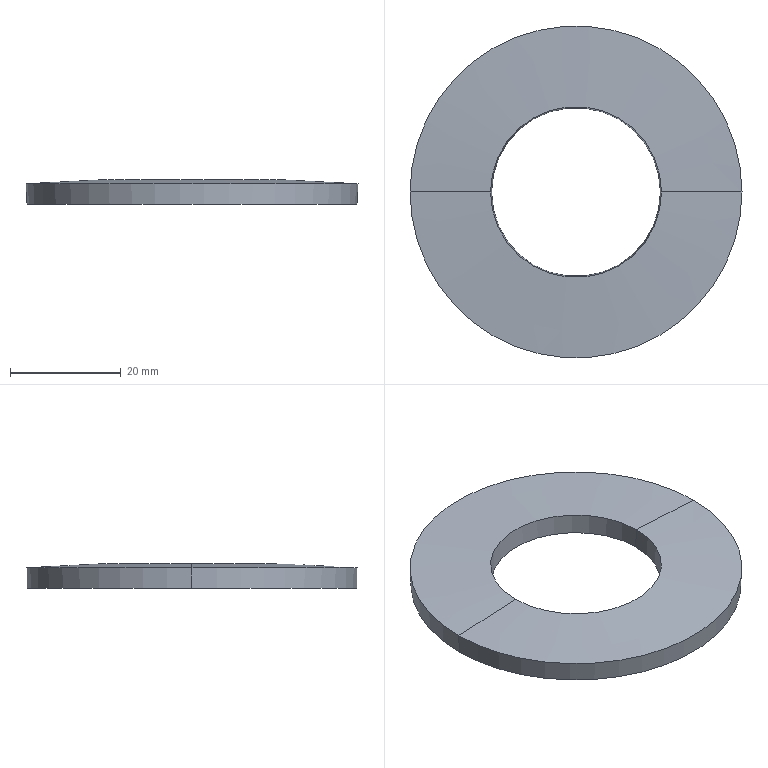Part | STEP file | PN_0065_default | 1 solid | 8 faces | box 60 x 60 x 4.5 mm | volume 7770 mm3 | cone 8
STEP:
#1=CARTESIAN_POINT('',(0.,0.,0.));
#2=DIRECTION('',(0.,0.,1.));
#3=DIRECTION('',(1.,0.,0.));
#4=AXIS2_PLACEMENT_3D('',#1,#2,#3);
#5=CARTESIAN_POINT('',(-15.25,0.,-2.045));
#6=VERTEX_POINT('',#5);
#7=CARTESIAN_POINT('',(-29.806,0.,-2.8));
#8=VERTEX_POINT('',#7);
#9=CARTESIAN_POINT('',(-29.806,0.,-2.8));
#10=DIRECTION('',(-0.9987,0.,-0.0518));
#11=VECTOR('',#10,1.);
#12=LINE('',#9,#11);
#13=CARTESIAN_POINT('',(0.,0.,-2.8));
#14=DIRECTION('',(0.,0.,-1.));
#15=DIRECTION('',(-1.,0.,0.));
#16=AXIS2_PLACEMENT_3D('',#13,#14,#15);
#17=CONICAL_SURFACE('',#16,29.806,1.519);
#18=CARTESIAN_POINT('',(6.283,0.));
#19=DIRECTION('',(0.,1.));
#20=VECTOR('',#19,1.);
#21=LINE('',#18,#20);
#22=(GEOMETRIC_REPRESENTATION_CONTEXT(2)PARAMETRIC_REPRESENTATION_CONTEXT()REPRESENTATION_CONTEXT('',''));
#23=DEFINITIONAL_REPRESENTATION('',(#21),#22);
#24=PCURVE('',#17,#23);
#25=CARTESIAN_POINT('',(0.,0.,-2.8));
#26=DIRECTION('',(0.,0.,-1.));
#27=DIRECTION('',(-1.,0.,0.));
#28=AXIS2_PLACEMENT_3D('',#25,#26,#27);
#29=CONICAL_SURFACE('',#28,29.806,1.519);
#30=CARTESIAN_POINT('',(0.,0.));
#31=DIRECTION('',(0.,1.));
#32=VECTOR('',#31,1.);
#33=LINE('',#30,#32);
#34=(GEOMETRIC_REPRESENTATION_CONTEXT(2)PARAMETRIC_REPRESENTATION_CONTEXT()REPRESENTATION_CONTEXT('',''));
#35=DEFINITIONAL_REPRESENTATION('',(#33),#34);
#36=PCURVE('',#29,#35);
#37=SURFACE_CURVE('',#12,(#24,#36),.PCURVE_S1.);
#38=EDGE_CURVE('',#6,#8,#37,.T.);
#39=ORIENTED_EDGE('',*,*,#38,.T.);
#40=CARTESIAN_POINT('',(29.806,0.,-2.8));
#41=VERTEX_POINT('',#40);
#42=CARTESIAN_POINT('',(0.,0.,-2.8));
#43=DIRECTION('',(0.,0.,1.));
#44=DIRECTION('',(1.,0.,0.));
#45=AXIS2_PLACEMENT_3D('',#42,#43,#44);
#46=CIRCLE('',#45,29.806);
#47=CARTESIAN_POINT('',(9.425,0.));
#48=DIRECTION('',(-1.,0.));
#49=VECTOR('',#48,1.);
#50=LINE('',#47,#49);
#51=(GEOMETRIC_REPRESENTATION_CONTEXT(2)PARAMETRIC_REPRESENTATION_CONTEXT()REPRESENTATION_CONTEXT('',''));
#52=DEFINITIONAL_REPRESENTATION('',(#50),#51);
#53=PCURVE('',#17,#52);
#54=CARTESIAN_POINT('',(0.,0.,0.945));
#55=DIRECTION('',(0.,0.,1.));
#56=DIRECTION('',(1.,0.,0.));
#57=AXIS2_PLACEMENT_3D('',#54,#55,#56);
#58=CONICAL_SURFACE('',#57,30.,0.05183);
#59=CARTESIAN_POINT('',(0.,-3.745));
#60=DIRECTION('',(1.,0.));
#61=VECTOR('',#60,1.);
#62=LINE('',#59,#61);
#63=(GEOMETRIC_REPRESENTATION_CONTEXT(2)PARAMETRIC_REPRESENTATION_CONTEXT()REPRESENTATION_CONTEXT('',''));
#64=DEFINITIONAL_REPRESENTATION('',(#62),#63);
#65=PCURVE('',#58,#64);
#66=SURFACE_CURVE('',#46,(#53,#65),.PCURVE_S1.);
#67=EDGE_CURVE('',#8,#41,#66,.T.);
#68=ORIENTED_EDGE('',*,*,#67,.T.);
#69=CARTESIAN_POINT('',(15.25,0.,-2.045));
#70=VERTEX_POINT('',#69);
#71=CARTESIAN_POINT('',(29.806,0.,-2.8));
#72=DIRECTION('',(0.9987,0.,-0.0518));
#73=VECTOR('',#72,1.);
#74=LINE('',#71,#73);
#75=CARTESIAN_POINT('',(3.142,0.));
#76=DIRECTION('',(0.,1.));
#77=VECTOR('',#76,1.);
#78=LINE('',#75,#77);
#79=(GEOMETRIC_REPRESENTATION_CONTEXT(2)PARAMETRIC_REPRESENTATION_CONTEXT()REPRESENTATION_CONTEXT('',''));
#80=DEFINITIONAL_REPRESENTATION('',(#78),#79);
#81=PCURVE('',#17,#80);
#82=CARTESIAN_POINT('',(3.142,0.));
#83=DIRECTION('',(0.,1.));
#84=VECTOR('',#83,1.);
#85=LINE('',#82,#84);
#86=(GEOMETRIC_REPRESENTATION_CONTEXT(2)PARAMETRIC_REPRESENTATION_CONTEXT()REPRESENTATION_CONTEXT('',''));
#87=DEFINITIONAL_REPRESENTATION('',(#85),#86);
#88=PCURVE('',#29,#87);
#89=SURFACE_CURVE('',#74,(#81,#88),.PCURVE_S1.);
#90=EDGE_CURVE('',#70,#41,#89,.T.);
#91=ORIENTED_EDGE('',*,*,#90,.F.);
#92=CARTESIAN_POINT('',(0.,0.,-2.045));
#93=DIRECTION('',(0.,0.,1.));
#94=DIRECTION('',(1.,0.,0.));
#95=AXIS2_PLACEMENT_3D('',#92,#93,#94);
#96=CIRCLE('',#95,15.25);
#97=CARTESIAN_POINT('',(9.425,-0.755));
#98=DIRECTION('',(-1.,0.));
#99=VECTOR('',#98,1.);
#100=LINE('',#97,#99);
#101=(GEOMETRIC_REPRESENTATION_CONTEXT(2)PARAMETRIC_REPRESENTATION_CONTEXT()REPRESENTATION_CONTEXT('',''));
#102=DEFINITIONAL_REPRESENTATION('',(#100),#101);
#103=PCURVE('',#17,#102);
#104=CARTESIAN_POINT('',(0.,0.,-2.045));
#105=DIRECTION('',(0.,0.,1.));
#106=DIRECTION('',(1.,0.,0.));
#107=AXIS2_PLACEMENT_3D('',#104,#105,#106);
#108=CONICAL_SURFACE('',#107,15.25,0.05183);
#109=CARTESIAN_POINT('',(0.,0.));
#110=DIRECTION('',(1.,0.));
#111=VECTOR('',#110,1.);
#112=LINE('',#109,#111);
#113=(GEOMETRIC_REPRESENTATION_CONTEXT(2)PARAMETRIC_REPRESENTATION_CONTEXT()REPRESENTATION_CONTEXT('',''));
#114=DEFINITIONAL_REPRESENTATION('',(#112),#113);
#115=PCURVE('',#108,#114);
#116=SURFACE_CURVE('',#96,(#103,#115),.PCURVE_S1.);
#117=EDGE_CURVE('',#6,#70,#116,.T.);
#118=ORIENTED_EDGE('',*,*,#117,.F.);
#119=EDGE_LOOP('',(#39,#68,#91,#118));
#120=FACE_BOUND('',#119,.F.);
#121=ADVANCED_FACE('',(#120),#17,.F.);
#122=CARTESIAN_POINT('',(0.,0.,-2.8));
#123=DIRECTION('',(0.,0.,1.));
#124=DIRECTION('',(1.,0.,0.));
#125=AXIS2_PLACEMENT_3D('',#122,#123,#124);
#126=CIRCLE('',#125,29.806);
#127=CARTESIAN_POINT('',(0.,0.,0.945));
#128=DIRECTION('',(0.,0.,1.));
#129=DIRECTION('',(1.,0.,0.));
#130=AXIS2_PLACEMENT_3D('',#127,#128,#129);
#131=CONICAL_SURFACE('',#130,30.,0.05183);
#132=CARTESIAN_POINT('',(0.,-3.745));
#133=DIRECTION('',(1.,0.));
#134=VECTOR('',#133,1.);
#135=LINE('',#132,#134);
#136=(GEOMETRIC_REPRESENTATION_CONTEXT(2)PARAMETRIC_REPRESENTATION_CONTEXT()REPRESENTATION_CONTEXT('',''));
#137=DEFINITIONAL_REPRESENTATION('',(#135),#136);
#138=PCURVE('',#131,#137);
#139=CARTESIAN_POINT('',(3.142,0.));
#140=DIRECTION('',(-1.,0.));
#141=VECTOR('',#140,1.);
#142=LINE('',#139,#141);
#143=(GEOMETRIC_REPRESENTATION_CONTEXT(2)PARAMETRIC_REPRESENTATION_CONTEXT()REPRESENTATION_CONTEXT('',''));
#144=DEFINITIONAL_REPRESENTATION('',(#142),#143);
#145=PCURVE('',#29,#144);
#146=SURFACE_CURVE('',#126,(#138,#145),.PCURVE_S1.);
#147=EDGE_CURVE('',#41,#8,#146,.T.);
#148=ORIENTED_EDGE('',*,*,#147,.T.);
#149=CARTESIAN_POINT('',(-30.,0.,0.945));
#150=VERTEX_POINT('',#149);
#151=CARTESIAN_POINT('',(-30.,0.,0.945));
#152=DIRECTION('',(-0.0518,0.,0.9987));
#153=VECTOR('',#152,1.);
#154=LINE('',#151,#153);
#155=CARTESIAN_POINT('',(3.142,0.));
#156=DIRECTION('',(0.,1.));
#157=VECTOR('',#156,1.);
#158=LINE('',#155,#157);
#159=(GEOMETRIC_REPRESENTATION_CONTEXT(2)PARAMETRIC_REPRESENTATION_CONTEXT()REPRESENTATION_CONTEXT('',''));
#160=DEFINITIONAL_REPRESENTATION('',(#158),#159);
#161=PCURVE('',#131,#160);
#162=CARTESIAN_POINT('',(3.142,0.));
#163=DIRECTION('',(0.,1.));
#164=VECTOR('',#163,1.);
#165=LINE('',#162,#164);
#166=(GEOMETRIC_REPRESENTATION_CONTEXT(2)PARAMETRIC_REPRESENTATION_CONTEXT()REPRESENTATION_CONTEXT('',''));
#167=DEFINITIONAL_REPRESENTATION('',(#165),#166);
#168=PCURVE('',#58,#167);
#169=SURFACE_CURVE('',#154,(#161,#168),.PCURVE_S1.);
#170=EDGE_CURVE('',#8,#150,#169,.T.);
#171=ORIENTED_EDGE('',*,*,#170,.T.);
#172=CARTESIAN_POINT('',(30.,0.,0.945));
#173=VERTEX_POINT('',#172);
#174=CARTESIAN_POINT('',(0.,0.,0.945));
#175=DIRECTION('',(0.,0.,1.));
#176=DIRECTION('',(1.,0.,0.));
#177=AXIS2_PLACEMENT_3D('',#174,#175,#176);
#178=CIRCLE('',#177,30.);
#179=CARTESIAN_POINT('',(0.,0.));
#180=DIRECTION('',(1.,0.));
#181=VECTOR('',#180,1.);
#182=LINE('',#179,#181);
#183=(GEOMETRIC_REPRESENTATION_CONTEXT(2)PARAMETRIC_REPRESENTATION_CONTEXT()REPRESENTATION_CONTEXT('',''));
#184=DEFINITIONAL_REPRESENTATION('',(#182),#183);
#185=PCURVE('',#131,#184);
#186=CARTESIAN_POINT('',(0.,0.,1.7));
#187=DIRECTION('',(0.,0.,-1.));
#188=DIRECTION('',(-1.,0.,0.));
#189=AXIS2_PLACEMENT_3D('',#186,#187,#188);
#190=CONICAL_SURFACE('',#189,15.444,1.519);
#191=CARTESIAN_POINT('',(3.142,0.755));
#192=DIRECTION('',(-1.,0.));
#193=VECTOR('',#192,1.);
#194=LINE('',#191,#193);
#195=(GEOMETRIC_REPRESENTATION_CONTEXT(2)PARAMETRIC_REPRESENTATION_CONTEXT()REPRESENTATION_CONTEXT('',''));
#196=DEFINITIONAL_REPRESENTATION('',(#194),#195);
#197=PCURVE('',#190,#196);
#198=SURFACE_CURVE('',#178,(#185,#197),.PCURVE_S1.);
#199=EDGE_CURVE('',#173,#150,#198,.T.);
#200=ORIENTED_EDGE('',*,*,#199,.F.);
#201=CARTESIAN_POINT('',(30.,0.,0.945));
#202=DIRECTION('',(0.0518,0.,0.9987));
#203=VECTOR('',#202,1.);
#204=LINE('',#201,#203);
#205=CARTESIAN_POINT('',(0.,0.));
#206=DIRECTION('',(0.,1.));
#207=VECTOR('',#206,1.);
#208=LINE('',#205,#207);
#209=(GEOMETRIC_REPRESENTATION_CONTEXT(2)PARAMETRIC_REPRESENTATION_CONTEXT()REPRESENTATION_CONTEXT('',''));
#210=DEFINITIONAL_REPRESENTATION('',(#208),#209);
#211=PCURVE('',#131,#210);
#212=CARTESIAN_POINT('',(6.283,0.));
#213=DIRECTION('',(0.,1.));
#214=VECTOR('',#213,1.);
#215=LINE('',#212,#214);
#216=(GEOMETRIC_REPRESENTATION_CONTEXT(2)PARAMETRIC_REPRESENTATION_CONTEXT()REPRESENTATION_CONTEXT('',''));
#217=DEFINITIONAL_REPRESENTATION('',(#215),#216);
#218=PCURVE('',#58,#217);
#219=SURFACE_CURVE('',#204,(#211,#218),.PCURVE_S1.);
#220=EDGE_CURVE('',#41,#173,#219,.T.);
#221=ORIENTED_EDGE('',*,*,#220,.F.);
#222=EDGE_LOOP('',(#148,#171,#200,#221));
#223=FACE_BOUND('',#222,.T.);
#224=ADVANCED_FACE('',(#223),#131,.T.);
#225=CARTESIAN_POINT('',(15.444,0.,1.7));
#226=VERTEX_POINT('',#225);
#227=CARTESIAN_POINT('',(-15.444,0.,1.7));
#228=VERTEX_POINT('',#227);
#229=CARTESIAN_POINT('',(0.,0.,1.7));
#230=DIRECTION('',(0.,0.,1.));
#231=DIRECTION('',(1.,0.,0.));
#232=AXIS2_PLACEMENT_3D('',#229,#230,#231);
#233=CIRCLE('',#232,15.444);
#234=CARTESIAN_POINT('',(3.142,0.));
#235=DIRECTION('',(-1.,0.));
#236=VECTOR('',#235,1.);
#237=LINE('',#234,#236);
#238=(GEOMETRIC_REPRESENTATION_CONTEXT(2)PARAMETRIC_REPRESENTATION_CONTEXT()REPRESENTATION_CONTEXT('',''));
#239=DEFINITIONAL_REPRESENTATION('',(#237),#238);
#240=PCURVE('',#190,#239);
#241=CARTESIAN_POINT('',(0.,0.,-2.045));
#242=DIRECTION('',(0.,0.,1.));
#243=DIRECTION('',(1.,0.,0.));
#244=AXIS2_PLACEMENT_3D('',#241,#242,#243);
#245=CONICAL_SURFACE('',#244,15.25,0.05183);
#246=CARTESIAN_POINT('',(0.,3.745));
#247=DIRECTION('',(1.,0.));
#248=VECTOR('',#247,1.);
#249=LINE('',#246,#248);
#250=(GEOMETRIC_REPRESENTATION_CONTEXT(2)PARAMETRIC_REPRESENTATION_CONTEXT()REPRESENTATION_CONTEXT('',''));
#251=DEFINITIONAL_REPRESENTATION('',(#249),#250);
#252=PCURVE('',#245,#251);
#253=SURFACE_CURVE('',#233,(#240,#252),.PCURVE_S1.);
#254=EDGE_CURVE('',#226,#228,#253,.T.);
#255=ORIENTED_EDGE('',*,*,#254,.F.);
#256=CARTESIAN_POINT('',(15.444,0.,1.7));
#257=DIRECTION('',(0.9987,0.,-0.0518));
#258=VECTOR('',#257,1.);
#259=LINE('',#256,#258);
#260=CARTESIAN_POINT('',(3.142,0.));
#261=DIRECTION('',(0.,1.));
#262=VECTOR('',#261,1.);
#263=LINE('',#260,#262);
#264=(GEOMETRIC_REPRESENTATION_CONTEXT(2)PARAMETRIC_REPRESENTATION_CONTEXT()REPRESENTATION_CONTEXT('',''));
#265=DEFINITIONAL_REPRESENTATION('',(#263),#264);
#266=PCURVE('',#190,#265);
#267=CARTESIAN_POINT('',(0.,0.,1.7));
#268=DIRECTION('',(0.,0.,-1.));
#269=DIRECTION('',(-1.,0.,0.));
#270=AXIS2_PLACEMENT_3D('',#267,#268,#269);
#271=CONICAL_SURFACE('',#270,15.444,1.519);
#272=CARTESIAN_POINT('',(3.142,0.));
#273=DIRECTION('',(0.,1.));
#274=VECTOR('',#273,1.);
#275=LINE('',#272,#274);
#276=(GEOMETRIC_REPRESENTATION_CONTEXT(2)PARAMETRIC_REPRESENTATION_CONTEXT()REPRESENTATION_CONTEXT('',''));
#277=DEFINITIONAL_REPRESENTATION('',(#275),#276);
#278=PCURVE('',#271,#277);
#279=SURFACE_CURVE('',#259,(#266,#278),.PCURVE_S1.);
#280=EDGE_CURVE('',#226,#173,#279,.T.);
#281=ORIENTED_EDGE('',*,*,#280,.T.);
#282=ORIENTED_EDGE('',*,*,#199,.T.);
#283=CARTESIAN_POINT('',(-15.444,0.,1.7));
#284=DIRECTION('',(-0.9987,0.,-0.0518));
#285=VECTOR('',#284,1.);
#286=LINE('',#283,#285);
#287=CARTESIAN_POINT('',(0.,0.));
#288=DIRECTION('',(0.,1.));
#289=VECTOR('',#288,1.);
#290=LINE('',#287,#289);
#291=(GEOMETRIC_REPRESENTATION_CONTEXT(2)PARAMETRIC_REPRESENTATION_CONTEXT()REPRESENTATION_CONTEXT('',''));
#292=DEFINITIONAL_REPRESENTATION('',(#290),#291);
#293=PCURVE('',#190,#292);
#294=CARTESIAN_POINT('',(6.283,0.));
#295=DIRECTION('',(0.,1.));
#296=VECTOR('',#295,1.);
#297=LINE('',#294,#296);
#298=(GEOMETRIC_REPRESENTATION_CONTEXT(2)PARAMETRIC_REPRESENTATION_CONTEXT()REPRESENTATION_CONTEXT('',''));
#299=DEFINITIONAL_REPRESENTATION('',(#297),#298);
#300=PCURVE('',#271,#299);
#301=SURFACE_CURVE('',#286,(#293,#300),.PCURVE_S1.);
#302=EDGE_CURVE('',#228,#150,#301,.T.);
#303=ORIENTED_EDGE('',*,*,#302,.F.);
#304=EDGE_LOOP('',(#255,#281,#282,#303));
#305=FACE_BOUND('',#304,.T.);
#306=ADVANCED_FACE('',(#305),#190,.T.);
#307=CARTESIAN_POINT('',(15.25,0.,-2.045));
#308=DIRECTION('',(0.0518,0.,0.9987));
#309=VECTOR('',#308,1.);
#310=LINE('',#307,#309);
#311=CARTESIAN_POINT('',(6.283,0.));
#312=DIRECTION('',(0.,1.));
#313=VECTOR('',#312,1.);
#314=LINE('',#311,#313);
#315=(GEOMETRIC_REPRESENTATION_CONTEXT(2)PARAMETRIC_REPRESENTATION_CONTEXT()REPRESENTATION_CONTEXT('',''));
#316=DEFINITIONAL_REPRESENTATION('',(#314),#315);
#317=PCURVE('',#108,#316);
#318=CARTESIAN_POINT('',(0.,0.));
#319=DIRECTION('',(0.,1.));
#320=VECTOR('',#319,1.);
#321=LINE('',#318,#320);
#322=(GEOMETRIC_REPRESENTATION_CONTEXT(2)PARAMETRIC_REPRESENTATION_CONTEXT()REPRESENTATION_CONTEXT('',''));
#323=DEFINITIONAL_REPRESENTATION('',(#321),#322);
#324=PCURVE('',#245,#323);
#325=SURFACE_CURVE('',#310,(#317,#324),.PCURVE_S1.);
#326=EDGE_CURVE('',#70,#226,#325,.T.);
#327=ORIENTED_EDGE('',*,*,#326,.T.);
#328=CARTESIAN_POINT('',(0.,0.,1.7));
#329=DIRECTION('',(0.,0.,1.));
#330=DIRECTION('',(1.,0.,0.));
#331=AXIS2_PLACEMENT_3D('',#328,#329,#330);
#332=CIRCLE('',#331,15.444);
#333=CARTESIAN_POINT('',(0.,3.745));
#334=DIRECTION('',(1.,0.));
#335=VECTOR('',#334,1.);
#336=LINE('',#333,#335);
#337=(GEOMETRIC_REPRESENTATION_CONTEXT(2)PARAMETRIC_REPRESENTATION_CONTEXT()REPRESENTATION_CONTEXT('',''));
#338=DEFINITIONAL_REPRESENTATION('',(#336),#337);
#339=PCURVE('',#108,#338);
#340=CARTESIAN_POINT('',(9.425,0.));
#341=DIRECTION('',(-1.,0.));
#342=VECTOR('',#341,1.);
#343=LINE('',#340,#342);
#344=(GEOMETRIC_REPRESENTATION_CONTEXT(2)PARAMETRIC_REPRESENTATION_CONTEXT()REPRESENTATION_CONTEXT('',''));
#345=DEFINITIONAL_REPRESENTATION('',(#343),#344);
#346=PCURVE('',#271,#345);
#347=SURFACE_CURVE('',#332,(#339,#346),.PCURVE_S1.);
#348=EDGE_CURVE('',#228,#226,#347,.T.);
#349=ORIENTED_EDGE('',*,*,#348,.F.);
#350=CARTESIAN_POINT('',(-15.25,0.,-2.045));
#351=DIRECTION('',(-0.0518,0.,0.9987));
#352=VECTOR('',#351,1.);
#353=LINE('',#350,#352);
#354=CARTESIAN_POINT('',(3.142,0.));
#355=DIRECTION('',(0.,1.));
#356=VECTOR('',#355,1.);
#357=LINE('',#354,#356);
#358=(GEOMETRIC_REPRESENTATION_CONTEXT(2)PARAMETRIC_REPRESENTATION_CONTEXT()REPRESENTATION_CONTEXT('',''));
#359=DEFINITIONAL_REPRESENTATION('',(#357),#358);
#360=PCURVE('',#108,#359);
#361=CARTESIAN_POINT('',(3.142,0.));
#362=DIRECTION('',(0.,1.));
#363=VECTOR('',#362,1.);
#364=LINE('',#361,#363);
#365=(GEOMETRIC_REPRESENTATION_CONTEXT(2)PARAMETRIC_REPRESENTATION_CONTEXT()REPRESENTATION_CONTEXT('',''));
#366=DEFINITIONAL_REPRESENTATION('',(#364),#365);
#367=PCURVE('',#245,#366);
#368=SURFACE_CURVE('',#353,(#360,#367),.PCURVE_S1.);
#369=EDGE_CURVE('',#6,#228,#368,.T.);
#370=ORIENTED_EDGE('',*,*,#369,.F.);
#371=ORIENTED_EDGE('',*,*,#117,.T.);
#372=EDGE_LOOP('',(#327,#349,#370,#371));
#373=FACE_BOUND('',#372,.F.);
#374=ADVANCED_FACE('',(#373),#108,.F.);
#375=ORIENTED_EDGE('',*,*,#254,.F.);
#376=ORIENTED_EDGE('',*,*,#326,.F.);
#377=CARTESIAN_POINT('',(0.,0.,-2.045));
#378=DIRECTION('',(0.,0.,1.));
#379=DIRECTION('',(1.,0.,0.));
#380=AXIS2_PLACEMENT_3D('',#377,#378,#379);
#381=CIRCLE('',#380,15.25);
#382=CARTESIAN_POINT('',(0.,0.));
#383=DIRECTION('',(1.,0.));
#384=VECTOR('',#383,1.);
#385=LINE('',#382,#384);
#386=(GEOMETRIC_REPRESENTATION_CONTEXT(2)PARAMETRIC_REPRESENTATION_CONTEXT()REPRESENTATION_CONTEXT('',''));
#387=DEFINITIONAL_REPRESENTATION('',(#385),#386);
#388=PCURVE('',#245,#387);
#389=CARTESIAN_POINT('',(3.142,-0.755));
#390=DIRECTION('',(-1.,0.));
#391=VECTOR('',#390,1.);
#392=LINE('',#389,#391);
#393=(GEOMETRIC_REPRESENTATION_CONTEXT(2)PARAMETRIC_REPRESENTATION_CONTEXT()REPRESENTATION_CONTEXT('',''));
#394=DEFINITIONAL_REPRESENTATION('',(#392),#393);
#395=PCURVE('',#29,#394);
#396=SURFACE_CURVE('',#381,(#388,#395),.PCURVE_S1.);
#397=EDGE_CURVE('',#70,#6,#396,.T.);
#398=ORIENTED_EDGE('',*,*,#397,.T.);
#399=ORIENTED_EDGE('',*,*,#369,.T.);
#400=EDGE_LOOP('',(#375,#376,#398,#399));
#401=FACE_BOUND('',#400,.F.);
#402=ADVANCED_FACE('',(#401),#245,.F.);
#403=ORIENTED_EDGE('',*,*,#280,.F.);
#404=ORIENTED_EDGE('',*,*,#348,.F.);
#405=ORIENTED_EDGE('',*,*,#302,.T.);
#406=CARTESIAN_POINT('',(0.,0.,0.945));
#407=DIRECTION('',(0.,0.,1.));
#408=DIRECTION('',(1.,0.,0.));
#409=AXIS2_PLACEMENT_3D('',#406,#407,#408);
#410=CIRCLE('',#409,30.);
#411=CARTESIAN_POINT('',(9.425,0.755));
#412=DIRECTION('',(-1.,0.));
#413=VECTOR('',#412,1.);
#414=LINE('',#411,#413);
#415=(GEOMETRIC_REPRESENTATION_CONTEXT(2)PARAMETRIC_REPRESENTATION_CONTEXT()REPRESENTATION_CONTEXT('',''));
#416=DEFINITIONAL_REPRESENTATION('',(#414),#415);
#417=PCURVE('',#271,#416);
#418=CARTESIAN_POINT('',(0.,0.));
#419=DIRECTION('',(1.,0.));
#420=VECTOR('',#419,1.);
#421=LINE('',#418,#420);
#422=(GEOMETRIC_REPRESENTATION_CONTEXT(2)PARAMETRIC_REPRESENTATION_CONTEXT()REPRESENTATION_CONTEXT('',''));
#423=DEFINITIONAL_REPRESENTATION('',(#421),#422);
#424=PCURVE('',#58,#423);
#425=SURFACE_CURVE('',#410,(#417,#424),.PCURVE_S1.);
#426=EDGE_CURVE('',#150,#173,#425,.T.);
#427=ORIENTED_EDGE('',*,*,#426,.T.);
#428=EDGE_LOOP('',(#403,#404,#405,#427));
#429=FACE_BOUND('',#428,.T.);
#430=ADVANCED_FACE('',(#429),#271,.T.);
#431=ORIENTED_EDGE('',*,*,#170,.F.);
#432=ORIENTED_EDGE('',*,*,#67,.T.);
#433=ORIENTED_EDGE('',*,*,#220,.T.);
#434=ORIENTED_EDGE('',*,*,#426,.F.);
#435=EDGE_LOOP('',(#431,#432,#433,#434));
#436=FACE_BOUND('',#435,.T.);
#437=ADVANCED_FACE('',(#436),#58,.T.);
#438=ORIENTED_EDGE('',*,*,#147,.T.);
#439=ORIENTED_EDGE('',*,*,#38,.F.);
#440=ORIENTED_EDGE('',*,*,#397,.F.);
#441=ORIENTED_EDGE('',*,*,#90,.T.);
#442=EDGE_LOOP('',(#438,#439,#440,#441));
#443=FACE_BOUND('',#442,.F.);
#444=ADVANCED_FACE('',(#443),#29,.F.);
#445=CLOSED_SHELL('',(#121,#224,#306,#374,#402,#430,#437,#444));
#446=MANIFOLD_SOLID_BREP('',#445);
#447=(LENGTH_UNIT()NAMED_UNIT(*)SI_UNIT(.MILLI.,.METRE.));
#448=UNCERTAINTY_MEASURE_WITH_UNIT(LENGTH_MEASURE(0.0000001),#447,'','');
#449=(NAMED_UNIT(*)PLANE_ANGLE_UNIT()SI_UNIT($,.RADIAN.));
#450=(NAMED_UNIT(*)SI_UNIT($,.STERADIAN.)SOLID_ANGLE_UNIT());
#451=(GEOMETRIC_REPRESENTATION_CONTEXT(3)GLOBAL_UNCERTAINTY_ASSIGNED_CONTEXT((#448))GLOBAL_UNIT_ASSIGNED_CONTEXT((#447,#449,#450))REPRESENTATION_CONTEXT('',''));
#452=ADVANCED_BREP_SHAPE_REPRESENTATION('',(#4,#446),#451);